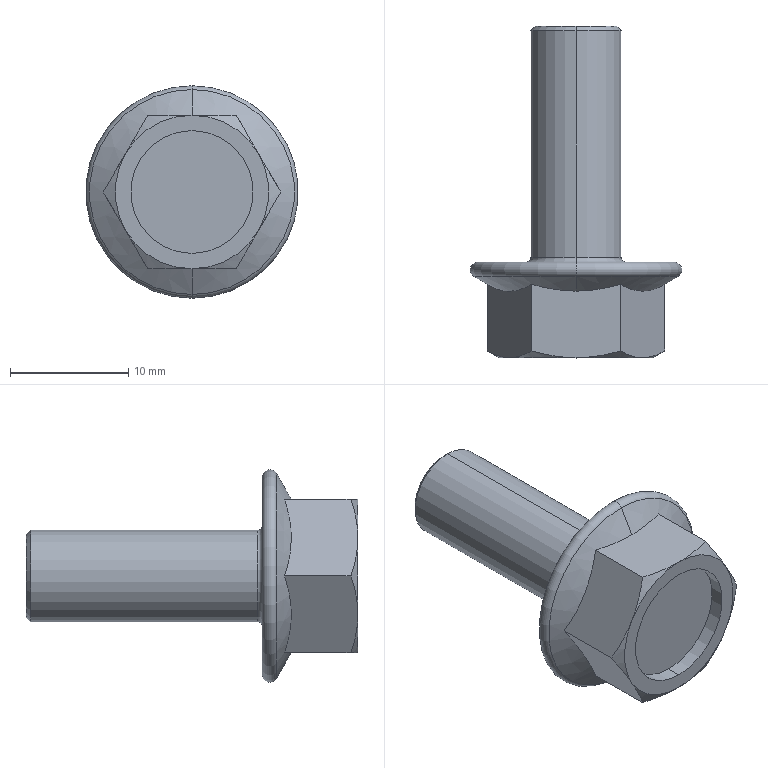Part | SolidWorks | features BaseBody 1 | 1 solid | 28 faces | box 18 x 28.1 x 18 mm | volume 2194 mm3 | cone 10 | plane 10 | torus 4 | cylinder 4 | commonest cylinder face diameters 7.76 x2 10.4 x2
STEP:
#1=CARTESIAN_POINT('',(198.,-222.95,186.322));
#2=VERTEX_POINT('',#1);
#3=CARTESIAN_POINT('',(198.,-222.95,203.678));
#4=VERTEX_POINT('',#3);
#5=CARTESIAN_POINT('',(198.,-222.95,195.));
#6=DIRECTION('',(0.,1.,0.));
#7=DIRECTION('',(0.,0.,-1.));
#8=AXIS2_PLACEMENT_3D('',#5,#6,#7);
#9=CIRCLE('',#8,8.678);
#10=EDGE_CURVE('',#2,#4,#9,.T.);
#11=ORIENTED_EDGE('',*,*,#10,.T.);
#12=CARTESIAN_POINT('',(198.,-221.75,203.357));
#13=VERTEX_POINT('',#12);
#14=CARTESIAN_POINT('',(198.,-222.393,203.357));
#15=DIRECTION('',(-1.,0.,0.));
#16=DIRECTION('',(0.,0.,1.));
#17=AXIS2_PLACEMENT_3D('',#14,#15,#16);
#18=CIRCLE('',#17,0.6431);
#19=EDGE_CURVE('',#4,#13,#18,.T.);
#20=ORIENTED_EDGE('',*,*,#19,.T.);
#21=CARTESIAN_POINT('',(198.,-221.75,186.643));
#22=VERTEX_POINT('',#21);
#23=CARTESIAN_POINT('',(198.,-221.75,195.));
#24=DIRECTION('',(0.,1.,0.));
#25=DIRECTION('',(0.,0.,-1.));
#26=AXIS2_PLACEMENT_3D('',#23,#24,#25);
#27=CIRCLE('',#26,8.357);
#28=EDGE_CURVE('',#22,#13,#27,.T.);
#29=ORIENTED_EDGE('',*,*,#28,.F.);
#30=CARTESIAN_POINT('',(198.,-222.393,186.643));
#31=DIRECTION('',(1.,0.,0.));
#32=DIRECTION('',(0.,0.,-1.));
#33=AXIS2_PLACEMENT_3D('',#30,#31,#32);
#34=CIRCLE('',#33,0.6431);
#35=EDGE_CURVE('',#2,#22,#34,.T.);
#36=ORIENTED_EDGE('',*,*,#35,.F.);
#37=EDGE_LOOP('',(#11,#20,#29,#36));
#38=FACE_OUTER_BOUND('',#37,.T.);
#39=CARTESIAN_POINT('',(198.,-222.393,195.));
#40=DIRECTION('',(0.,1.,0.));
#41=DIRECTION('',(0.,0.,-1.));
#42=AXIS2_PLACEMENT_3D('',#39,#40,#41);
#43=TOROIDAL_SURFACE('',#42,8.357,0.6431);
#44=ADVANCED_FACE('',(#38),#43,.T.);
#45=CARTESIAN_POINT('',(194.247,-223.627,201.5));
#46=VERTEX_POINT('',#45);
#47=CARTESIAN_POINT('',(198.,-224.208,201.5));
#48=VERTEX_POINT('',#47);
#49=CARTESIAN_POINT('',(194.247,-223.627,201.5));
#50=CARTESIAN_POINT('',(194.861,-223.804,201.5));
#51=CARTESIAN_POINT('',(195.48,-223.95,201.5));
#52=CARTESIAN_POINT('',(196.729,-224.152,201.5));
#53=CARTESIAN_POINT('',(197.361,-224.208,201.5));
#54=CARTESIAN_POINT('',(198.,-224.208,201.5));
#55=B_SPLINE_CURVE_WITH_KNOTS('',3,(#49,#50,#51,#52,#53,#54),.UNSPECIFIED.,.F.,.F.,(4,2,4),(0.,0.001899,0.003797),.UNSPECIFIED.);
#56=EDGE_CURVE('',#46,#48,#55,.T.);
#57=ORIENTED_EDGE('',*,*,#56,.T.);
#58=CARTESIAN_POINT('',(198.,-222.95,203.678));
#59=DIRECTION('',(0.,0.5,0.866));
#60=VECTOR('',#59,1000.);
#61=LINE('',#58,#60);
#62=EDGE_CURVE('',#48,#4,#61,.T.);
#63=ORIENTED_EDGE('',*,*,#62,.T.);
#64=ORIENTED_EDGE('',*,*,#10,.F.);
#65=CARTESIAN_POINT('',(198.,-224.208,188.5));
#66=VERTEX_POINT('',#65);
#67=CARTESIAN_POINT('',(198.,-222.95,186.322));
#68=DIRECTION('',(0.,0.5,-0.866));
#69=VECTOR('',#68,1000.);
#70=LINE('',#67,#69);
#71=EDGE_CURVE('',#66,#2,#70,.T.);
#72=ORIENTED_EDGE('',*,*,#71,.F.);
#73=CARTESIAN_POINT('',(194.247,-223.627,188.5));
#74=VERTEX_POINT('',#73);
#75=CARTESIAN_POINT('',(198.,-224.208,188.5));
#76=CARTESIAN_POINT('',(197.682,-224.208,188.5));
#77=CARTESIAN_POINT('',(197.362,-224.194,188.5));
#78=CARTESIAN_POINT('',(196.729,-224.141,188.5));
#79=CARTESIAN_POINT('',(196.414,-224.102,188.5));
#80=CARTESIAN_POINT('',(195.477,-223.95,188.5));
#81=CARTESIAN_POINT('',(194.86,-223.804,188.5));
#82=CARTESIAN_POINT('',(194.247,-223.627,188.5));
#83=B_SPLINE_CURVE_WITH_KNOTS('',3,(#75,#76,#77,#78,#79,#80,#81,#82),.UNSPECIFIED.,.F.,.F.,(4,2,2,4),(0.003797,0.004743,0.005689,0.00758),.UNSPECIFIED.);
#84=EDGE_CURVE('',#66,#74,#83,.T.);
#85=ORIENTED_EDGE('',*,*,#84,.T.);
#86=CARTESIAN_POINT('',(190.494,-223.627,195.));
#87=VERTEX_POINT('',#86);
#88=CARTESIAN_POINT('',(194.247,-223.627,188.5));
#89=CARTESIAN_POINT('',(193.941,-223.804,189.031));
#90=CARTESIAN_POINT('',(193.632,-223.95,189.565));
#91=CARTESIAN_POINT('',(193.009,-224.152,190.645));
#92=CARTESIAN_POINT('',(192.693,-224.207,191.191));
#93=CARTESIAN_POINT('',(192.215,-224.208,192.02));
#94=CARTESIAN_POINT('',(192.055,-224.194,192.298));
#95=CARTESIAN_POINT('',(191.738,-224.141,192.847));
#96=CARTESIAN_POINT('',(191.58,-224.102,193.12));
#97=CARTESIAN_POINT('',(191.111,-223.95,193.933));
#98=CARTESIAN_POINT('',(190.801,-223.804,194.469));
#99=CARTESIAN_POINT('',(190.494,-223.627,195.));
#100=B_SPLINE_CURVE_WITH_KNOTS('',3,(#88,#89,#90,#91,#92,#93,#94,#95,#96,#97,#98,#99),.UNSPECIFIED.,.F.,.F.,(4,2,2,2,2,4),(0.,0.001895,0.00379,0.004738,0.005685,0.00758),.UNSPECIFIED.);
#101=EDGE_CURVE('',#74,#87,#100,.T.);
#102=ORIENTED_EDGE('',*,*,#101,.T.);
#103=CARTESIAN_POINT('',(190.494,-223.627,195.));
#104=CARTESIAN_POINT('',(190.801,-223.804,195.531));
#105=CARTESIAN_POINT('',(191.109,-223.95,196.065));
#106=CARTESIAN_POINT('',(191.733,-224.152,197.145));
#107=CARTESIAN_POINT('',(192.048,-224.207,197.691));
#108=CARTESIAN_POINT('',(192.527,-224.208,198.52));
#109=CARTESIAN_POINT('',(192.687,-224.194,198.798));
#110=CARTESIAN_POINT('',(193.004,-224.141,199.347));
#111=CARTESIAN_POINT('',(193.162,-224.102,199.62));
#112=CARTESIAN_POINT('',(193.631,-223.95,200.433));
#113=CARTESIAN_POINT('',(193.94,-223.804,200.969));
#114=CARTESIAN_POINT('',(194.247,-223.627,201.5));
#115=B_SPLINE_CURVE_WITH_KNOTS('',3,(#103,#104,#105,#106,#107,#108,#109,#110,#111,#112,#113,#114),.UNSPECIFIED.,.F.,.F.,(4,2,2,2,2,4),(0.,0.001895,0.00379,0.004738,0.005685,0.00758),.UNSPECIFIED.);
#116=EDGE_CURVE('',#87,#46,#115,.T.);
#117=ORIENTED_EDGE('',*,*,#116,.T.);
#118=EDGE_LOOP('',(#57,#63,#64,#72,#85,#102,#117));
#119=FACE_OUTER_BOUND('',#118,.T.);
#120=CARTESIAN_POINT('',(198.,-222.95,195.));
#121=DIRECTION('',(0.,1.,0.));
#122=DIRECTION('',(0.,0.,-1.));
#123=AXIS2_PLACEMENT_3D('',#120,#121,#122);
#124=CONICAL_SURFACE('',#123,8.678,1.047);
#125=ADVANCED_FACE('',(#119),#124,.T.);
#126=CARTESIAN_POINT('',(198.,-202.138,198.88));
#127=VERTEX_POINT('',#126);
#128=CARTESIAN_POINT('',(198.,-202.138,191.12));
#129=VERTEX_POINT('',#128);
#130=CARTESIAN_POINT('',(198.,-202.138,195.));
#131=DIRECTION('',(0.,-1.,0.));
#132=DIRECTION('',(0.,0.,-1.));
#133=AXIS2_PLACEMENT_3D('',#130,#131,#132);
#134=CIRCLE('',#133,3.88);
#135=EDGE_CURVE('',#127,#129,#134,.T.);
#136=ORIENTED_EDGE('',*,*,#135,.T.);
#137=CARTESIAN_POINT('',(198.,-221.35,191.12));
#138=VERTEX_POINT('',#137);
#139=CARTESIAN_POINT('',(198.,-201.75,191.12));
#140=DIRECTION('',(0.,-1.,0.));
#141=VECTOR('',#140,1000.);
#142=LINE('',#139,#141);
#143=EDGE_CURVE('',#129,#138,#142,.T.);
#144=ORIENTED_EDGE('',*,*,#143,.T.);
#145=CARTESIAN_POINT('',(198.,-221.35,198.88));
#146=VERTEX_POINT('',#145);
#147=CARTESIAN_POINT('',(198.,-221.35,195.));
#148=DIRECTION('',(0.,1.,0.));
#149=DIRECTION('',(0.,0.,-1.));
#150=AXIS2_PLACEMENT_3D('',#147,#148,#149);
#151=CIRCLE('',#150,3.88);
#152=EDGE_CURVE('',#138,#146,#151,.T.);
#153=ORIENTED_EDGE('',*,*,#152,.T.);
#154=CARTESIAN_POINT('',(198.,-201.75,198.88));
#155=DIRECTION('',(0.,-1.,0.));
#156=VECTOR('',#155,1000.);
#157=LINE('',#154,#156);
#158=EDGE_CURVE('',#127,#146,#157,.T.);
#159=ORIENTED_EDGE('',*,*,#158,.F.);
#160=EDGE_LOOP('',(#136,#144,#153,#159));
#161=FACE_OUTER_BOUND('',#160,.T.);
#162=CARTESIAN_POINT('',(198.,-201.75,195.));
#163=DIRECTION('',(0.,-1.,0.));
#164=DIRECTION('',(0.,0.,1.));
#165=AXIS2_PLACEMENT_3D('',#162,#163,#164);
#166=CYLINDRICAL_SURFACE('',#165,3.88);
#167=ADVANCED_FACE('',(#161),#166,.T.);
#168=CARTESIAN_POINT('',(198.,-229.85,200.2));
#169=VERTEX_POINT('',#168);
#170=CARTESIAN_POINT('',(198.,-229.85,189.8));
#171=VERTEX_POINT('',#170);
#172=CARTESIAN_POINT('',(198.,-229.85,195.));
#173=DIRECTION('',(0.,1.,0.));
#174=DIRECTION('',(0.,0.,1.));
#175=AXIS2_PLACEMENT_3D('',#172,#173,#174);
#176=CIRCLE('',#175,5.2);
#177=EDGE_CURVE('',#169,#171,#176,.T.);
#178=ORIENTED_EDGE('',*,*,#177,.F.);
#179=CARTESIAN_POINT('',(198.,-228.635,200.2));
#180=VERTEX_POINT('',#179);
#181=CARTESIAN_POINT('',(198.,-229.85,200.2));
#182=DIRECTION('',(0.,1.,0.));
#183=VECTOR('',#182,1000.);
#184=LINE('',#181,#183);
#185=EDGE_CURVE('',#169,#180,#184,.T.);
#186=ORIENTED_EDGE('',*,*,#185,.T.);
#187=CARTESIAN_POINT('',(198.,-228.635,189.8));
#188=VERTEX_POINT('',#187);
#189=CARTESIAN_POINT('',(198.,-228.635,195.));
#190=DIRECTION('',(0.,-1.,0.));
#191=DIRECTION('',(0.,0.,1.));
#192=AXIS2_PLACEMENT_3D('',#189,#190,#191);
#193=CIRCLE('',#192,5.2);
#194=EDGE_CURVE('',#188,#180,#193,.T.);
#195=ORIENTED_EDGE('',*,*,#194,.F.);
#196=CARTESIAN_POINT('',(198.,-229.85,189.8));
#197=DIRECTION('',(0.,1.,0.));
#198=VECTOR('',#197,1000.);
#199=LINE('',#196,#198);
#200=EDGE_CURVE('',#171,#188,#199,.T.);
#201=ORIENTED_EDGE('',*,*,#200,.F.);
#202=EDGE_LOOP('',(#178,#186,#195,#201));
#203=FACE_OUTER_BOUND('',#202,.T.);
#204=CARTESIAN_POINT('',(198.,-229.85,195.));
#205=DIRECTION('',(0.,1.,0.));
#206=DIRECTION('',(0.,0.,-1.));
#207=AXIS2_PLACEMENT_3D('',#204,#205,#206);
#208=CYLINDRICAL_SURFACE('',#207,5.2);
#209=ADVANCED_FACE('',(#203),#208,.F.);
#210=CARTESIAN_POINT('',(198.,-201.75,191.508));
#211=VERTEX_POINT('',#210);
#212=CARTESIAN_POINT('',(198.,-201.75,198.492));
#213=VERTEX_POINT('',#212);
#214=CARTESIAN_POINT('',(198.,-201.75,195.));
#215=DIRECTION('',(0.,1.,0.));
#216=DIRECTION('',(0.,0.,-1.));
#217=AXIS2_PLACEMENT_3D('',#214,#215,#216);
#218=CIRCLE('',#217,3.492);
#219=EDGE_CURVE('',#211,#213,#218,.T.);
#220=ORIENTED_EDGE('',*,*,#219,.F.);
#221=CARTESIAN_POINT('',(198.,-201.75,191.508));
#222=DIRECTION('',(0.,-0.7071,-0.7071));
#223=VECTOR('',#222,1000.);
#224=LINE('',#221,#223);
#225=EDGE_CURVE('',#211,#129,#224,.T.);
#226=ORIENTED_EDGE('',*,*,#225,.T.);
#227=ORIENTED_EDGE('',*,*,#135,.F.);
#228=CARTESIAN_POINT('',(198.,-201.75,198.492));
#229=DIRECTION('',(0.,-0.7071,0.7071));
#230=VECTOR('',#229,1000.);
#231=LINE('',#228,#230);
#232=EDGE_CURVE('',#213,#127,#231,.T.);
#233=ORIENTED_EDGE('',*,*,#232,.F.);
#234=EDGE_LOOP('',(#220,#226,#227,#233));
#235=FACE_OUTER_BOUND('',#234,.T.);
#236=CARTESIAN_POINT('',(198.,-201.75,195.));
#237=DIRECTION('',(0.,-1.,0.));
#238=DIRECTION('',(0.,0.,1.));
#239=AXIS2_PLACEMENT_3D('',#236,#237,#238);
#240=CONICAL_SURFACE('',#239,3.492,0.7854);
#241=ADVANCED_FACE('',(#235),#240,.T.);
#242=CARTESIAN_POINT('',(198.,-221.35,195.));
#243=DIRECTION('',(0.,1.,0.));
#244=DIRECTION('',(0.,0.,-1.));
#245=AXIS2_PLACEMENT_3D('',#242,#243,#244);
#246=CIRCLE('',#245,3.88);
#247=EDGE_CURVE('',#146,#138,#246,.T.);
#248=ORIENTED_EDGE('',*,*,#247,.F.);
#249=CARTESIAN_POINT('',(198.,-221.75,199.28));
#250=VERTEX_POINT('',#249);
#251=CARTESIAN_POINT('',(198.,-221.35,199.28));
#252=DIRECTION('',(-1.,0.,0.));
#253=DIRECTION('',(0.,0.,1.));
#254=AXIS2_PLACEMENT_3D('',#251,#252,#253);
#255=CIRCLE('',#254,0.4);
#256=EDGE_CURVE('',#146,#250,#255,.T.);
#257=ORIENTED_EDGE('',*,*,#256,.T.);
#258=CARTESIAN_POINT('',(198.,-221.75,190.72));
#259=VERTEX_POINT('',#258);
#260=CARTESIAN_POINT('',(198.,-221.75,195.));
#261=DIRECTION('',(0.,-1.,0.));
#262=DIRECTION('',(0.,0.,-1.));
#263=AXIS2_PLACEMENT_3D('',#260,#261,#262);
#264=CIRCLE('',#263,4.28);
#265=EDGE_CURVE('',#259,#250,#264,.T.);
#266=ORIENTED_EDGE('',*,*,#265,.F.);
#267=CARTESIAN_POINT('',(198.,-221.35,190.72));
#268=DIRECTION('',(1.,0.,0.));
#269=DIRECTION('',(0.,0.,-1.));
#270=AXIS2_PLACEMENT_3D('',#267,#268,#269);
#271=CIRCLE('',#270,0.4);
#272=EDGE_CURVE('',#138,#259,#271,.T.);
#273=ORIENTED_EDGE('',*,*,#272,.F.);
#274=EDGE_LOOP('',(#248,#257,#266,#273));
#275=FACE_OUTER_BOUND('',#274,.T.);
#276=CARTESIAN_POINT('',(198.,-221.35,195.));
#277=DIRECTION('',(0.,1.,0.));
#278=DIRECTION('',(0.,0.,-1.));
#279=AXIS2_PLACEMENT_3D('',#276,#277,#278);
#280=TOROIDAL_SURFACE('',#279,4.28,0.4);
#281=ADVANCED_FACE('',(#275),#280,.F.);
#282=ORIENTED_EDGE('',*,*,#256,.F.);
#283=ORIENTED_EDGE('',*,*,#152,.F.);
#284=ORIENTED_EDGE('',*,*,#272,.T.);
#285=CARTESIAN_POINT('',(198.,-221.75,195.));
#286=DIRECTION('',(0.,-1.,0.));
#287=DIRECTION('',(0.,0.,-1.));
#288=AXIS2_PLACEMENT_3D('',#285,#286,#287);
#289=CIRCLE('',#288,4.28);
#290=EDGE_CURVE('',#250,#259,#289,.T.);
#291=ORIENTED_EDGE('',*,*,#290,.F.);
#292=EDGE_LOOP('',(#282,#283,#284,#291));
#293=FACE_OUTER_BOUND('',#292,.T.);
#294=CARTESIAN_POINT('',(198.,-221.35,195.));
#295=DIRECTION('',(0.,1.,0.));
#296=DIRECTION('',(0.,0.,-1.));
#297=AXIS2_PLACEMENT_3D('',#294,#295,#296);
#298=TOROIDAL_SURFACE('',#297,4.28,0.4);
#299=ADVANCED_FACE('',(#293),#298,.F.);
#300=ORIENTED_EDGE('',*,*,#225,.F.);
#301=CARTESIAN_POINT('',(198.,-201.75,195.));
#302=DIRECTION('',(0.,1.,0.));
#303=DIRECTION('',(0.,0.,-1.));
#304=AXIS2_PLACEMENT_3D('',#301,#302,#303);
#305=CIRCLE('',#304,3.492);
#306=EDGE_CURVE('',#213,#211,#305,.T.);
#307=ORIENTED_EDGE('',*,*,#306,.F.);
#308=ORIENTED_EDGE('',*,*,#232,.T.);
#309=CARTESIAN_POINT('',(198.,-202.138,195.));
#310=DIRECTION('',(0.,-1.,0.));
#311=DIRECTION('',(0.,0.,-1.));
#312=AXIS2_PLACEMENT_3D('',#309,#310,#311);
#313=CIRCLE('',#312,3.88);
#314=EDGE_CURVE('',#129,#127,#313,.T.);
#315=ORIENTED_EDGE('',*,*,#314,.F.);
#316=EDGE_LOOP('',(#300,#307,#308,#315));
#317=FACE_OUTER_BOUND('',#316,.T.);
#318=CARTESIAN_POINT('',(198.,-201.75,195.));
#319=DIRECTION('',(0.,-1.,0.));
#320=DIRECTION('',(0.,0.,1.));
#321=AXIS2_PLACEMENT_3D('',#318,#319,#320);
#322=CONICAL_SURFACE('',#321,3.492,0.7854);
#323=ADVANCED_FACE('',(#317),#322,.T.);
#324=CARTESIAN_POINT('',(198.,-229.85,188.5));
#325=VERTEX_POINT('',#324);
#326=CARTESIAN_POINT('',(192.371,-229.85,191.75));
#327=VERTEX_POINT('',#326);
#328=CARTESIAN_POINT('',(198.,-229.85,195.));
#329=DIRECTION('',(0.,1.,0.));
#330=DIRECTION('',(0.,0.,-1.));
#331=AXIS2_PLACEMENT_3D('',#328,#329,#330);
#332=CIRCLE('',#331,6.5);
#333=EDGE_CURVE('',#325,#327,#332,.T.);
#334=ORIENTED_EDGE('',*,*,#333,.F.);
#335=CARTESIAN_POINT('',(203.629,-229.85,191.75));
#336=VERTEX_POINT('',#335);
#337=CARTESIAN_POINT('',(198.,-229.85,195.));
#338=DIRECTION('',(0.,1.,0.));
#339=DIRECTION('',(0.,0.,-1.));
#340=AXIS2_PLACEMENT_3D('',#337,#338,#339);
#341=CIRCLE('',#340,6.5);
#342=EDGE_CURVE('',#336,#325,#341,.T.);
#343=ORIENTED_EDGE('',*,*,#342,.F.);
#344=CARTESIAN_POINT('',(203.629,-229.85,198.25));
#345=VERTEX_POINT('',#344);
#346=CARTESIAN_POINT('',(198.,-229.85,195.));
#347=DIRECTION('',(0.,1.,0.));
#348=DIRECTION('',(0.,0.,-1.));
#349=AXIS2_PLACEMENT_3D('',#346,#347,#348);
#350=CIRCLE('',#349,6.5);
#351=EDGE_CURVE('',#345,#336,#350,.T.);
#352=ORIENTED_EDGE('',*,*,#351,.F.);
#353=CARTESIAN_POINT('',(198.,-229.85,201.5));
#354=VERTEX_POINT('',#353);
#355=CARTESIAN_POINT('',(198.,-229.85,195.));
#356=DIRECTION('',(0.,1.,0.));
#357=DIRECTION('',(0.,0.,-1.));
#358=AXIS2_PLACEMENT_3D('',#355,#356,#357);
#359=CIRCLE('',#358,6.5);
#360=EDGE_CURVE('',#354,#345,#359,.T.);
#361=ORIENTED_EDGE('',*,*,#360,.F.);
#362=CARTESIAN_POINT('',(192.371,-229.85,198.25));
#363=VERTEX_POINT('',#362);
#364=CARTESIAN_POINT('',(198.,-229.85,195.));
#365=DIRECTION('',(0.,1.,0.));
#366=DIRECTION('',(0.,0.,-1.));
#367=AXIS2_PLACEMENT_3D('',#364,#365,#366);
#368=CIRCLE('',#367,6.5);
#369=EDGE_CURVE('',#363,#354,#368,.T.);
#370=ORIENTED_EDGE('',*,*,#369,.F.);
#371=CARTESIAN_POINT('',(198.,-229.85,195.));
#372=DIRECTION('',(0.,1.,0.));
#373=DIRECTION('',(0.,0.,-1.));
#374=AXIS2_PLACEMENT_3D('',#371,#372,#373);
#375=CIRCLE('',#374,6.5);
#376=EDGE_CURVE('',#327,#363,#375,.T.);
#377=ORIENTED_EDGE('',*,*,#376,.F.);
#378=EDGE_LOOP('',(#334,#343,#352,#361,#370,#377));
#379=FACE_OUTER_BOUND('',#378,.T.);
#380=CARTESIAN_POINT('',(198.,-229.85,195.));
#381=DIRECTION('',(0.,1.,0.));
#382=DIRECTION('',(0.,0.,1.));
#383=AXIS2_PLACEMENT_3D('',#380,#381,#382);
#384=CIRCLE('',#383,5.2);
#385=EDGE_CURVE('',#171,#169,#384,.T.);
#386=ORIENTED_EDGE('',*,*,#385,.T.);
#387=ORIENTED_EDGE('',*,*,#177,.T.);
#388=EDGE_LOOP('',(#386,#387));
#389=FACE_BOUND('',#388,.T.);
#390=CARTESIAN_POINT('',(194.247,-229.85,201.5));
#391=DIRECTION('',(0.,1.,0.));
#392=DIRECTION('',(1.,0.,0.));
#393=AXIS2_PLACEMENT_3D('',#390,#391,#392);
#394=PLANE('',#393);
#395=ADVANCED_FACE('',(#379,#389),#394,.F.);
#396=ORIENTED_EDGE('',*,*,#185,.F.);
#397=ORIENTED_EDGE('',*,*,#385,.F.);
#398=ORIENTED_EDGE('',*,*,#200,.T.);
#399=CARTESIAN_POINT('',(198.,-228.635,195.));
#400=DIRECTION('',(0.,-1.,0.));
#401=DIRECTION('',(0.,0.,1.));
#402=AXIS2_PLACEMENT_3D('',#399,#400,#401);
#403=CIRCLE('',#402,5.2);
#404=EDGE_CURVE('',#180,#188,#403,.T.);
#405=ORIENTED_EDGE('',*,*,#404,.F.);
#406=EDGE_LOOP('',(#396,#397,#398,#405));
#407=FACE_OUTER_BOUND('',#406,.T.);
#408=CARTESIAN_POINT('',(198.,-229.85,195.));
#409=DIRECTION('',(0.,1.,0.));
#410=DIRECTION('',(0.,0.,-1.));
#411=AXIS2_PLACEMENT_3D('',#408,#409,#410);
#412=CYLINDRICAL_SURFACE('',#411,5.2);
#413=ADVANCED_FACE('',(#407),#412,.F.);
#414=ORIENTED_EDGE('',*,*,#194,.T.);
#415=ORIENTED_EDGE('',*,*,#404,.T.);
#416=EDGE_LOOP('',(#414,#415));
#417=FACE_OUTER_BOUND('',#416,.T.);
#418=CARTESIAN_POINT('',(198.,-228.635,195.));
#419=DIRECTION('',(0.,1.,0.));
#420=DIRECTION('',(1.,0.,0.));
#421=AXIS2_PLACEMENT_3D('',#418,#419,#420);
#422=PLANE('',#421);
#423=ADVANCED_FACE('',(#417),#422,.F.);
#424=CARTESIAN_POINT('',(194.247,-229.269,201.5));
#425=VERTEX_POINT('',#424);
#426=CARTESIAN_POINT('',(198.,-229.85,201.5));
#427=CARTESIAN_POINT('',(196.719,-229.85,201.5));
#428=CARTESIAN_POINT('',(195.473,-229.623,201.5));
#429=CARTESIAN_POINT('',(194.247,-229.269,201.5));
#430=B_SPLINE_CURVE_WITH_KNOTS('',3,(#426,#427,#428,#429),.UNSPECIFIED.,.F.,.F.,(4,4),(0.,0.003797),.UNSPECIFIED.);
#431=EDGE_CURVE('',#354,#425,#430,.T.);
#432=ORIENTED_EDGE('',*,*,#431,.T.);
#433=CARTESIAN_POINT('',(194.247,-229.269,201.5));
#434=CARTESIAN_POINT('',(193.634,-229.623,200.438));
#435=CARTESIAN_POINT('',(193.011,-229.85,199.359));
#436=CARTESIAN_POINT('',(192.371,-229.85,198.25));
#437=B_SPLINE_CURVE_WITH_KNOTS('',3,(#433,#434,#435,#436),.UNSPECIFIED.,.F.,.F.,(4,4),(0.,0.003797),.UNSPECIFIED.);
#438=EDGE_CURVE('',#425,#363,#437,.T.);
#439=ORIENTED_EDGE('',*,*,#438,.T.);
#440=ORIENTED_EDGE('',*,*,#369,.T.);
#441=EDGE_LOOP('',(#432,#439,#440));
#442=FACE_OUTER_BOUND('',#441,.T.);
#443=CARTESIAN_POINT('',(198.,-229.85,195.));
#444=DIRECTION('',(0.,1.,0.));
#445=DIRECTION('',(0.,0.,-1.));
#446=AXIS2_PLACEMENT_3D('',#443,#444,#445);
#447=CONICAL_SURFACE('',#446,6.5,1.047);
#448=ADVANCED_FACE('',(#442),#447,.T.);
#449=CARTESIAN_POINT('',(201.753,-229.269,201.5));
#450=VERTEX_POINT('',#449);
#451=CARTESIAN_POINT('',(203.629,-229.85,198.25));
#452=CARTESIAN_POINT('',(202.989,-229.85,199.359));
#453=CARTESIAN_POINT('',(202.366,-229.623,200.438));
#454=CARTESIAN_POINT('',(201.753,-229.269,201.5));
#455=B_SPLINE_CURVE_WITH_KNOTS('',3,(#451,#452,#453,#454),.UNSPECIFIED.,.F.,.F.,(4,4),(0.,0.003797),.UNSPECIFIED.);
#456=EDGE_CURVE('',#345,#450,#455,.T.);
#457=ORIENTED_EDGE('',*,*,#456,.T.);
#458=CARTESIAN_POINT('',(201.753,-229.269,201.5));
#459=CARTESIAN_POINT('',(200.527,-229.623,201.5));
#460=CARTESIAN_POINT('',(199.281,-229.85,201.5));
#461=CARTESIAN_POINT('',(198.,-229.85,201.5));
#462=B_SPLINE_CURVE_WITH_KNOTS('',3,(#458,#459,#460,#461),.UNSPECIFIED.,.F.,.F.,(4,4),(0.,0.003797),.UNSPECIFIED.);
#463=EDGE_CURVE('',#450,#354,#462,.T.);
#464=ORIENTED_EDGE('',*,*,#463,.T.);
#465=ORIENTED_EDGE('',*,*,#360,.T.);
#466=EDGE_LOOP('',(#457,#464,#465));
#467=FACE_OUTER_BOUND('',#466,.T.);
#468=CARTESIAN_POINT('',(198.,-229.85,195.));
#469=DIRECTION('',(0.,1.,0.));
#470=DIRECTION('',(0.,0.,-1.));
#471=AXIS2_PLACEMENT_3D('',#468,#469,#470);
#472=CONICAL_SURFACE('',#471,6.5,1.047);
#473=ADVANCED_FACE('',(#467),#472,.T.);
#474=CARTESIAN_POINT('',(205.506,-229.269,195.));
#475=VERTEX_POINT('',#474);
#476=CARTESIAN_POINT('',(205.506,-229.269,195.));
#477=CARTESIAN_POINT('',(204.892,-229.623,196.062));
#478=CARTESIAN_POINT('',(204.27,-229.85,197.141));
#479=CARTESIAN_POINT('',(203.629,-229.85,198.25));
#480=B_SPLINE_CURVE_WITH_KNOTS('',3,(#476,#477,#478,#479),.UNSPECIFIED.,.F.,.F.,(4,4),(0.,0.003797),.UNSPECIFIED.);
#481=EDGE_CURVE('',#475,#345,#480,.T.);
#482=ORIENTED_EDGE('',*,*,#481,.T.);
#483=ORIENTED_EDGE('',*,*,#351,.T.);
#484=CARTESIAN_POINT('',(203.629,-229.85,191.75));
#485=CARTESIAN_POINT('',(204.27,-229.85,192.859));
#486=CARTESIAN_POINT('',(204.892,-229.623,193.938));
#487=CARTESIAN_POINT('',(205.506,-229.269,195.));
#488=B_SPLINE_CURVE_WITH_KNOTS('',3,(#484,#485,#486,#487),.UNSPECIFIED.,.F.,.F.,(4,4),(0.,0.003797),.UNSPECIFIED.);
#489=EDGE_CURVE('',#336,#475,#488,.T.);
#490=ORIENTED_EDGE('',*,*,#489,.T.);
#491=EDGE_LOOP('',(#482,#483,#490));
#492=FACE_OUTER_BOUND('',#491,.T.);
#493=CARTESIAN_POINT('',(198.,-229.85,195.));
#494=DIRECTION('',(0.,1.,0.));
#495=DIRECTION('',(0.,0.,-1.));
#496=AXIS2_PLACEMENT_3D('',#493,#494,#495);
#497=CONICAL_SURFACE('',#496,6.5,1.047);
#498=ADVANCED_FACE('',(#492),#497,.T.);
#499=CARTESIAN_POINT('',(201.753,-229.269,188.5));
#500=VERTEX_POINT('',#499);
#501=CARTESIAN_POINT('',(201.753,-229.269,188.5));
#502=CARTESIAN_POINT('',(202.366,-229.623,189.562));
#503=CARTESIAN_POINT('',(202.989,-229.85,190.641));
#504=CARTESIAN_POINT('',(203.629,-229.85,191.75));
#505=B_SPLINE_CURVE_WITH_KNOTS('',3,(#501,#502,#503,#504),.UNSPECIFIED.,.F.,.F.,(4,4),(0.,0.003797),.UNSPECIFIED.);
#506=EDGE_CURVE('',#500,#336,#505,.T.);
#507=ORIENTED_EDGE('',*,*,#506,.T.);
#508=ORIENTED_EDGE('',*,*,#342,.T.);
#509=CARTESIAN_POINT('',(198.,-229.85,188.5));
#510=CARTESIAN_POINT('',(199.281,-229.85,188.5));
#511=CARTESIAN_POINT('',(200.527,-229.623,188.5));
#512=CARTESIAN_POINT('',(201.753,-229.269,188.5));
#513=B_SPLINE_CURVE_WITH_KNOTS('',3,(#509,#510,#511,#512),.UNSPECIFIED.,.F.,.F.,(4,4),(0.,0.003797),.UNSPECIFIED.);
#514=EDGE_CURVE('',#325,#500,#513,.T.);
#515=ORIENTED_EDGE('',*,*,#514,.T.);
#516=EDGE_LOOP('',(#507,#508,#515));
#517=FACE_OUTER_BOUND('',#516,.T.);
#518=CARTESIAN_POINT('',(198.,-229.85,195.));
#519=DIRECTION('',(0.,1.,0.));
#520=DIRECTION('',(0.,0.,-1.));
#521=AXIS2_PLACEMENT_3D('',#518,#519,#520);
#522=CONICAL_SURFACE('',#521,6.5,1.047);
#523=ADVANCED_FACE('',(#517),#522,.T.);
#524=CARTESIAN_POINT('',(190.494,-229.269,195.));
#525=VERTEX_POINT('',#524);
#526=CARTESIAN_POINT('',(192.371,-229.85,198.25));
#527=CARTESIAN_POINT('',(191.73,-229.85,197.141));
#528=CARTESIAN_POINT('',(191.108,-229.623,196.062));
#529=CARTESIAN_POINT('',(190.494,-229.269,195.));
#530=B_SPLINE_CURVE_WITH_KNOTS('',3,(#526,#527,#528,#529),.UNSPECIFIED.,.F.,.F.,(4,4),(0.,0.003797),.UNSPECIFIED.);
#531=EDGE_CURVE('',#363,#525,#530,.T.);
#532=ORIENTED_EDGE('',*,*,#531,.T.);
#533=CARTESIAN_POINT('',(190.494,-229.269,195.));
#534=CARTESIAN_POINT('',(191.108,-229.623,193.938));
#535=CARTESIAN_POINT('',(191.73,-229.85,192.859));
#536=CARTESIAN_POINT('',(192.371,-229.85,191.75));
#537=B_SPLINE_CURVE_WITH_KNOTS('',3,(#533,#534,#535,#536),.UNSPECIFIED.,.F.,.F.,(4,4),(0.,0.003797),.UNSPECIFIED.);
#538=EDGE_CURVE('',#525,#327,#537,.T.);
#539=ORIENTED_EDGE('',*,*,#538,.T.);
#540=ORIENTED_EDGE('',*,*,#376,.T.);
#541=EDGE_LOOP('',(#532,#539,#540));
#542=FACE_OUTER_BOUND('',#541,.T.);
#543=CARTESIAN_POINT('',(198.,-229.85,195.));
#544=DIRECTION('',(0.,1.,0.));
#545=DIRECTION('',(0.,0.,-1.));
#546=AXIS2_PLACEMENT_3D('',#543,#544,#545);
#547=CONICAL_SURFACE('',#546,6.5,1.047);
#548=ADVANCED_FACE('',(#542),#547,.T.);
#549=CARTESIAN_POINT('',(194.247,-229.269,188.5));
#550=VERTEX_POINT('',#549);
#551=CARTESIAN_POINT('',(194.247,-229.269,188.5));
#552=CARTESIAN_POINT('',(195.473,-229.623,188.5));
#553=CARTESIAN_POINT('',(196.719,-229.85,188.5));
#554=CARTESIAN_POINT('',(198.,-229.85,188.5));
#555=B_SPLINE_CURVE_WITH_KNOTS('',3,(#551,#552,#553,#554),.UNSPECIFIED.,.F.,.F.,(4,4),(0.,0.003797),.UNSPECIFIED.);
#556=EDGE_CURVE('',#550,#325,#555,.T.);
#557=ORIENTED_EDGE('',*,*,#556,.T.);
#558=ORIENTED_EDGE('',*,*,#333,.T.);
#559=CARTESIAN_POINT('',(192.371,-229.85,191.75));
#560=CARTESIAN_POINT('',(193.011,-229.85,190.641));
#561=CARTESIAN_POINT('',(193.634,-229.623,189.562));
#562=CARTESIAN_POINT('',(194.247,-229.269,188.5));
#563=B_SPLINE_CURVE_WITH_KNOTS('',3,(#559,#560,#561,#562),.UNSPECIFIED.,.F.,.F.,(4,4),(0.,0.003797),.UNSPECIFIED.);
#564=EDGE_CURVE('',#327,#550,#563,.T.);
#565=ORIENTED_EDGE('',*,*,#564,.T.);
#566=EDGE_LOOP('',(#557,#558,#565));
#567=FACE_OUTER_BOUND('',#566,.T.);
#568=CARTESIAN_POINT('',(198.,-229.85,195.));
#569=DIRECTION('',(0.,1.,0.));
#570=DIRECTION('',(0.,0.,-1.));
#571=AXIS2_PLACEMENT_3D('',#568,#569,#570);
#572=CONICAL_SURFACE('',#571,6.5,1.047);
#573=ADVANCED_FACE('',(#567),#572,.T.);
#574=ORIENTED_EDGE('',*,*,#306,.T.);
#575=ORIENTED_EDGE('',*,*,#219,.T.);
#576=EDGE_LOOP('',(#574,#575));
#577=FACE_OUTER_BOUND('',#576,.T.);
#578=CARTESIAN_POINT('',(198.,-201.75,195.));
#579=DIRECTION('',(0.,1.,0.));
#580=DIRECTION('',(1.,0.,0.));
#581=AXIS2_PLACEMENT_3D('',#578,#579,#580);
#582=PLANE('',#581);
#583=ADVANCED_FACE('',(#577),#582,.T.);
#584=ORIENTED_EDGE('',*,*,#143,.F.);
#585=ORIENTED_EDGE('',*,*,#314,.T.);
#586=ORIENTED_EDGE('',*,*,#158,.T.);
#587=ORIENTED_EDGE('',*,*,#247,.T.);
#588=EDGE_LOOP('',(#584,#585,#586,#587));
#589=FACE_OUTER_BOUND('',#588,.T.);
#590=CARTESIAN_POINT('',(198.,-201.75,195.));
#591=DIRECTION('',(0.,-1.,0.));
#592=DIRECTION('',(0.,0.,1.));
#593=AXIS2_PLACEMENT_3D('',#590,#591,#592);
#594=CYLINDRICAL_SURFACE('',#593,3.88);
#595=ADVANCED_FACE('',(#589),#594,.T.);
#596=ORIENTED_EDGE('',*,*,#28,.T.);
#597=CARTESIAN_POINT('',(198.,-221.75,195.));
#598=DIRECTION('',(0.,1.,0.));
#599=DIRECTION('',(0.,0.,-1.));
#600=AXIS2_PLACEMENT_3D('',#597,#598,#599);
#601=CIRCLE('',#600,8.357);
#602=EDGE_CURVE('',#13,#22,#601,.T.);
#603=ORIENTED_EDGE('',*,*,#602,.T.);
#604=EDGE_LOOP('',(#596,#603));
#605=FACE_OUTER_BOUND('',#604,.T.);
#606=ORIENTED_EDGE('',*,*,#265,.T.);
#607=ORIENTED_EDGE('',*,*,#290,.T.);
#608=EDGE_LOOP('',(#606,#607));
#609=FACE_BOUND('',#608,.T.);
#610=CARTESIAN_POINT('',(194.247,-221.75,201.5));
#611=DIRECTION('',(0.,1.,0.));
#612=DIRECTION('',(1.,0.,0.));
#613=AXIS2_PLACEMENT_3D('',#610,#611,#612);
#614=PLANE('',#613);
#615=ADVANCED_FACE('',(#605,#609),#614,.T.);
#616=ORIENTED_EDGE('',*,*,#62,.F.);
#617=CARTESIAN_POINT('',(201.753,-223.627,201.5));
#618=VERTEX_POINT('',#617);
#619=CARTESIAN_POINT('',(198.,-224.208,201.5));
#620=CARTESIAN_POINT('',(198.318,-224.208,201.5));
#621=CARTESIAN_POINT('',(198.638,-224.194,201.5));
#622=CARTESIAN_POINT('',(199.271,-224.141,201.5));
#623=CARTESIAN_POINT('',(199.586,-224.102,201.5));
#624=CARTESIAN_POINT('',(200.523,-223.95,201.5));
#625=CARTESIAN_POINT('',(201.14,-223.804,201.5));
#626=CARTESIAN_POINT('',(201.753,-223.627,201.5));
#627=B_SPLINE_CURVE_WITH_KNOTS('',3,(#619,#620,#621,#622,#623,#624,#625,#626),.UNSPECIFIED.,.F.,.F.,(4,2,2,4),(0.003797,0.004743,0.005689,0.00758),.UNSPECIFIED.);
#628=EDGE_CURVE('',#48,#618,#627,.T.);
#629=ORIENTED_EDGE('',*,*,#628,.T.);
#630=CARTESIAN_POINT('',(205.506,-223.627,195.));
#631=VERTEX_POINT('',#630);
#632=CARTESIAN_POINT('',(201.753,-223.627,201.5));
#633=CARTESIAN_POINT('',(202.059,-223.804,200.969));
#634=CARTESIAN_POINT('',(202.368,-223.95,200.435));
#635=CARTESIAN_POINT('',(202.991,-224.152,199.355));
#636=CARTESIAN_POINT('',(203.307,-224.207,198.809));
#637=CARTESIAN_POINT('',(203.785,-224.208,197.98));
#638=CARTESIAN_POINT('',(203.945,-224.194,197.702));
#639=CARTESIAN_POINT('',(204.262,-224.141,197.153));
#640=CARTESIAN_POINT('',(204.42,-224.102,196.88));
#641=CARTESIAN_POINT('',(204.889,-223.95,196.067));
#642=CARTESIAN_POINT('',(205.199,-223.804,195.531));
#643=CARTESIAN_POINT('',(205.506,-223.627,195.));
#644=B_SPLINE_CURVE_WITH_KNOTS('',3,(#632,#633,#634,#635,#636,#637,#638,#639,#640,#641,#642,#643),.UNSPECIFIED.,.F.,.F.,(4,2,2,2,2,4),(0.,0.001895,0.00379,0.004738,0.005685,0.00758),.UNSPECIFIED.);
#645=EDGE_CURVE('',#618,#631,#644,.T.);
#646=ORIENTED_EDGE('',*,*,#645,.T.);
#647=CARTESIAN_POINT('',(201.753,-223.627,188.5));
#648=VERTEX_POINT('',#647);
#649=CARTESIAN_POINT('',(205.506,-223.627,195.));
#650=CARTESIAN_POINT('',(205.199,-223.804,194.469));
#651=CARTESIAN_POINT('',(204.891,-223.95,193.935));
#652=CARTESIAN_POINT('',(204.267,-224.152,192.855));
#653=CARTESIAN_POINT('',(203.952,-224.207,192.309));
#654=CARTESIAN_POINT('',(203.473,-224.208,191.48));
#655=CARTESIAN_POINT('',(203.313,-224.194,191.202));
#656=CARTESIAN_POINT('',(202.996,-224.141,190.653));
#657=CARTESIAN_POINT('',(202.838,-224.102,190.38));
#658=CARTESIAN_POINT('',(202.369,-223.95,189.567));
#659=CARTESIAN_POINT('',(202.06,-223.804,189.031));
#660=CARTESIAN_POINT('',(201.753,-223.627,188.5));
#661=B_SPLINE_CURVE_WITH_KNOTS('',3,(#649,#650,#651,#652,#653,#654,#655,#656,#657,#658,#659,#660),.UNSPECIFIED.,.F.,.F.,(4,2,2,2,2,4),(0.,0.001895,0.00379,0.004738,0.005685,0.00758),.UNSPECIFIED.);
#662=EDGE_CURVE('',#631,#648,#661,.T.);
#663=ORIENTED_EDGE('',*,*,#662,.T.);
#664=CARTESIAN_POINT('',(201.753,-223.627,188.5));
#665=CARTESIAN_POINT('',(201.139,-223.804,188.5));
#666=CARTESIAN_POINT('',(200.52,-223.95,188.5));
#667=CARTESIAN_POINT('',(199.271,-224.152,188.5));
#668=CARTESIAN_POINT('',(198.639,-224.208,188.5));
#669=CARTESIAN_POINT('',(198.,-224.208,188.5));
#670=B_SPLINE_CURVE_WITH_KNOTS('',3,(#664,#665,#666,#667,#668,#669),.UNSPECIFIED.,.F.,.F.,(4,2,4),(0.,0.001899,0.003797),.UNSPECIFIED.);
#671=EDGE_CURVE('',#648,#66,#670,.T.);
#672=ORIENTED_EDGE('',*,*,#671,.T.);
#673=ORIENTED_EDGE('',*,*,#71,.T.);
#674=CARTESIAN_POINT('',(198.,-222.95,195.));
#675=DIRECTION('',(0.,1.,0.));
#676=DIRECTION('',(0.,0.,-1.));
#677=AXIS2_PLACEMENT_3D('',#674,#675,#676);
#678=CIRCLE('',#677,8.678);
#679=EDGE_CURVE('',#4,#2,#678,.T.);
#680=ORIENTED_EDGE('',*,*,#679,.F.);
#681=EDGE_LOOP('',(#616,#629,#646,#663,#672,#673,#680));
#682=FACE_OUTER_BOUND('',#681,.T.);
#683=CARTESIAN_POINT('',(198.,-222.95,195.));
#684=DIRECTION('',(0.,1.,0.));
#685=DIRECTION('',(0.,0.,-1.));
#686=AXIS2_PLACEMENT_3D('',#683,#684,#685);
#687=CONICAL_SURFACE('',#686,8.678,1.047);
#688=ADVANCED_FACE('',(#682),#687,.T.);
#689=ORIENTED_EDGE('',*,*,#19,.F.);
#690=ORIENTED_EDGE('',*,*,#679,.T.);
#691=ORIENTED_EDGE('',*,*,#35,.T.);
#692=ORIENTED_EDGE('',*,*,#602,.F.);
#693=EDGE_LOOP('',(#689,#690,#691,#692));
#694=FACE_OUTER_BOUND('',#693,.T.);
#695=CARTESIAN_POINT('',(198.,-222.393,195.));
#696=DIRECTION('',(0.,1.,0.));
#697=DIRECTION('',(0.,0.,-1.));
#698=AXIS2_PLACEMENT_3D('',#695,#696,#697);
#699=TOROIDAL_SURFACE('',#698,8.357,0.6431);
#700=ADVANCED_FACE('',(#694),#699,.T.);
#701=ORIENTED_EDGE('',*,*,#538,.F.);
#702=CARTESIAN_POINT('',(190.494,-229.85,195.));
#703=DIRECTION('',(0.,1.,0.));
#704=VECTOR('',#703,1000.);
#705=LINE('',#702,#704);
#706=EDGE_CURVE('',#525,#87,#705,.T.);
#707=ORIENTED_EDGE('',*,*,#706,.T.);
#708=ORIENTED_EDGE('',*,*,#101,.F.);
#709=CARTESIAN_POINT('',(194.247,-229.85,188.5));
#710=DIRECTION('',(0.,1.,0.));
#711=VECTOR('',#710,1000.);
#712=LINE('',#709,#711);
#713=EDGE_CURVE('',#550,#74,#712,.T.);
#714=ORIENTED_EDGE('',*,*,#713,.F.);
#715=ORIENTED_EDGE('',*,*,#564,.F.);
#716=EDGE_LOOP('',(#701,#707,#708,#714,#715));
#717=FACE_OUTER_BOUND('',#716,.T.);
#718=CARTESIAN_POINT('',(194.247,-229.85,188.5));
#719=DIRECTION('',(-0.866,0.,-0.5));
#720=DIRECTION('',(-0.5,0.,0.866));
#721=AXIS2_PLACEMENT_3D('',#718,#719,#720);
#722=PLANE('',#721);
#723=ADVANCED_FACE('',(#717),#722,.T.);
#724=ORIENTED_EDGE('',*,*,#556,.F.);
#725=ORIENTED_EDGE('',*,*,#713,.T.);
#726=ORIENTED_EDGE('',*,*,#84,.F.);
#727=ORIENTED_EDGE('',*,*,#671,.F.);
#728=CARTESIAN_POINT('',(201.753,-229.85,188.5));
#729=DIRECTION('',(0.,1.,0.));
#730=VECTOR('',#729,1000.);
#731=LINE('',#728,#730);
#732=EDGE_CURVE('',#500,#648,#731,.T.);
#733=ORIENTED_EDGE('',*,*,#732,.F.);
#734=ORIENTED_EDGE('',*,*,#514,.F.);
#735=EDGE_LOOP('',(#724,#725,#726,#727,#733,#734));
#736=FACE_OUTER_BOUND('',#735,.T.);
#737=CARTESIAN_POINT('',(201.753,-229.85,188.5));
#738=DIRECTION('',(0.,0.,-1.));
#739=DIRECTION('',(0.,-1.,0.));
#740=AXIS2_PLACEMENT_3D('',#737,#738,#739);
#741=PLANE('',#740);
#742=ADVANCED_FACE('',(#736),#741,.T.);
#743=ORIENTED_EDGE('',*,*,#506,.F.);
#744=ORIENTED_EDGE('',*,*,#732,.T.);
#745=ORIENTED_EDGE('',*,*,#662,.F.);
#746=CARTESIAN_POINT('',(205.506,-229.85,195.));
#747=DIRECTION('',(0.,1.,0.));
#748=VECTOR('',#747,1000.);
#749=LINE('',#746,#748);
#750=EDGE_CURVE('',#475,#631,#749,.T.);
#751=ORIENTED_EDGE('',*,*,#750,.F.);
#752=ORIENTED_EDGE('',*,*,#489,.F.);
#753=EDGE_LOOP('',(#743,#744,#745,#751,#752));
#754=FACE_OUTER_BOUND('',#753,.T.);
#755=CARTESIAN_POINT('',(205.506,-229.85,195.));
#756=DIRECTION('',(0.866,0.,-0.5));
#757=DIRECTION('',(0.,-1.,0.));
#758=AXIS2_PLACEMENT_3D('',#755,#756,#757);
#759=PLANE('',#758);
#760=ADVANCED_FACE('',(#754),#759,.T.);
#761=ORIENTED_EDGE('',*,*,#481,.F.);
#762=ORIENTED_EDGE('',*,*,#750,.T.);
#763=ORIENTED_EDGE('',*,*,#645,.F.);
#764=CARTESIAN_POINT('',(201.753,-229.85,201.5));
#765=DIRECTION('',(0.,1.,0.));
#766=VECTOR('',#765,1000.);
#767=LINE('',#764,#766);
#768=EDGE_CURVE('',#450,#618,#767,.T.);
#769=ORIENTED_EDGE('',*,*,#768,.F.);
#770=ORIENTED_EDGE('',*,*,#456,.F.);
#771=EDGE_LOOP('',(#761,#762,#763,#769,#770));
#772=FACE_OUTER_BOUND('',#771,.T.);
#773=CARTESIAN_POINT('',(201.753,-229.85,201.5));
#774=DIRECTION('',(0.866,0.,0.5));
#775=DIRECTION('',(0.,-1.,0.));
#776=AXIS2_PLACEMENT_3D('',#773,#774,#775);
#777=PLANE('',#776);
#778=ADVANCED_FACE('',(#772),#777,.T.);
#779=ORIENTED_EDGE('',*,*,#463,.F.);
#780=ORIENTED_EDGE('',*,*,#768,.T.);
#781=ORIENTED_EDGE('',*,*,#628,.F.);
#782=ORIENTED_EDGE('',*,*,#56,.F.);
#783=CARTESIAN_POINT('',(194.247,-229.85,201.5));
#784=DIRECTION('',(0.,1.,0.));
#785=VECTOR('',#784,1000.);
#786=LINE('',#783,#785);
#787=EDGE_CURVE('',#425,#46,#786,.T.);
#788=ORIENTED_EDGE('',*,*,#787,.F.);
#789=ORIENTED_EDGE('',*,*,#431,.F.);
#790=EDGE_LOOP('',(#779,#780,#781,#782,#788,#789));
#791=FACE_OUTER_BOUND('',#790,.T.);
#792=CARTESIAN_POINT('',(194.247,-229.85,201.5));
#793=DIRECTION('',(0.,0.,1.));
#794=DIRECTION('',(1.,0.,0.));
#795=AXIS2_PLACEMENT_3D('',#792,#793,#794);
#796=PLANE('',#795);
#797=ADVANCED_FACE('',(#791),#796,.T.);
#798=ORIENTED_EDGE('',*,*,#438,.F.);
#799=ORIENTED_EDGE('',*,*,#787,.T.);
#800=ORIENTED_EDGE('',*,*,#116,.F.);
#801=ORIENTED_EDGE('',*,*,#706,.F.);
#802=ORIENTED_EDGE('',*,*,#531,.F.);
#803=EDGE_LOOP('',(#798,#799,#800,#801,#802));
#804=FACE_OUTER_BOUND('',#803,.T.);
#805=CARTESIAN_POINT('',(190.494,-229.85,195.));
#806=DIRECTION('',(-0.866,0.,0.5));
#807=DIRECTION('',(0.,1.,0.));
#808=AXIS2_PLACEMENT_3D('',#805,#806,#807);
#809=PLANE('',#808);
#810=ADVANCED_FACE('',(#804),#809,.T.);
#811=CLOSED_SHELL('',(#44,#125,#167,#209,#241,#281,#299,#323,#395,#413,#423,#448,#473,#498,#523,#548,#573,#583,#595,#615,#688,#700,#723,#742,#760,#778,#797,#810));
#812=MANIFOLD_SOLID_BREP('',#811);
#813=CARTESIAN_POINT('',(0.,0.,0.));
#814=DIRECTION('',(0.,0.,1.));
#815=DIRECTION('',(1.,0.,0.));
#816=AXIS2_PLACEMENT_3D('',#813,#814,#815);
#817=(LENGTH_UNIT()NAMED_UNIT(*)SI_UNIT(.MILLI.,.METRE.));
#818=UNCERTAINTY_MEASURE_WITH_UNIT(LENGTH_MEASURE(0.00001),#817,'','');
#819=(NAMED_UNIT(*)PLANE_ANGLE_UNIT()SI_UNIT($,.RADIAN.));
#820=(NAMED_UNIT(*)SI_UNIT($,.STERADIAN.)SOLID_ANGLE_UNIT());
#821=(GEOMETRIC_REPRESENTATION_CONTEXT(3)GLOBAL_UNCERTAINTY_ASSIGNED_CONTEXT((#818))GLOBAL_UNIT_ASSIGNED_CONTEXT((#817,#819,#820))REPRESENTATION_CONTEXT('',''));
#822=ADVANCED_BREP_SHAPE_REPRESENTATION('',(#812,#816),#821);